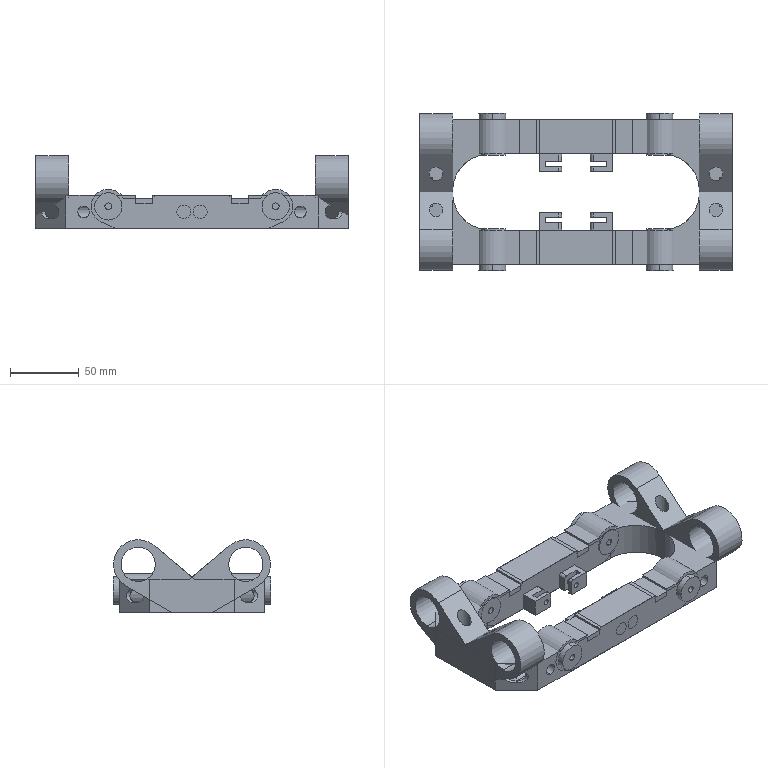Part | 4 solids | 302 faces | box 228 x 114.503 x 53 mm | volume 575344 mm3 | cylinder 170 | plane 132 | commonest cylinder face diameters 10 x46 3 x16 3.5 x16 4.1 x16 8.6 x16 20 x16